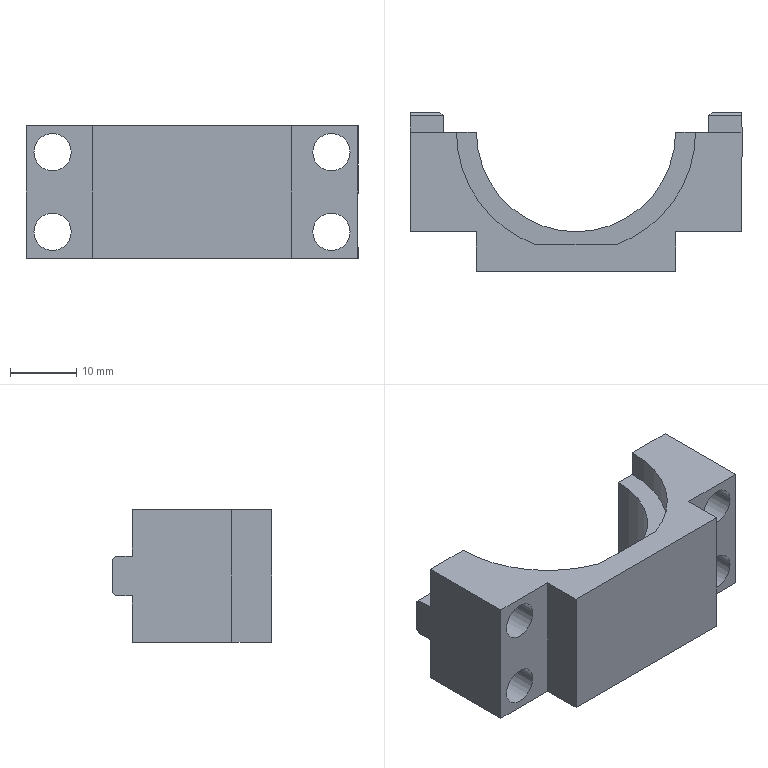Part | SolidWorks | features ICE 5, Chamfer 1, Extrusion 1 | 1 solid | 38 faces | box 50 x 24 x 20 mm | volume 9639 mm3 | plane 27 | cylinder 11 | commonest cylinder face diameters 5.6 x8 36 x2 30 x1
STEP:
#1=CARTESIAN_POINT('',(18.2,10.5,16.));
#2=VERTEX_POINT('',#1);
#3=CARTESIAN_POINT('',(23.8,10.5,16.));
#4=VERTEX_POINT('',#3);
#5=CARTESIAN_POINT('',(21.,10.5,16.));
#6=DIRECTION('',(0.,-1.,0.));
#7=DIRECTION('',(1.,0.,0.));
#8=AXIS2_PLACEMENT_3D('',#5,#6,#7);
#9=CIRCLE('',#8,2.8);
#10=EDGE_CURVE('',#2,#4,#9,.T.);
#11=ORIENTED_EDGE('',*,*,#10,.F.);
#12=CARTESIAN_POINT('',(18.2,-4.5,16.));
#13=VERTEX_POINT('',#12);
#14=CARTESIAN_POINT('',(18.2,15.5,16.));
#15=DIRECTION('',(0.,-1.,0.));
#16=VECTOR('',#15,1000.);
#17=LINE('',#14,#16);
#18=EDGE_CURVE('',#2,#13,#17,.T.);
#19=ORIENTED_EDGE('',*,*,#18,.T.);
#20=CARTESIAN_POINT('',(23.8,-4.5,16.));
#21=VERTEX_POINT('',#20);
#22=CARTESIAN_POINT('',(21.,-4.5,16.));
#23=DIRECTION('',(0.,-1.,0.));
#24=DIRECTION('',(1.,0.,0.));
#25=AXIS2_PLACEMENT_3D('',#22,#23,#24);
#26=CIRCLE('',#25,2.8);
#27=EDGE_CURVE('',#13,#21,#26,.T.);
#28=ORIENTED_EDGE('',*,*,#27,.T.);
#29=CARTESIAN_POINT('',(23.8,15.5,16.));
#30=DIRECTION('',(0.,-1.,0.));
#31=VECTOR('',#30,1000.);
#32=LINE('',#29,#31);
#33=EDGE_CURVE('',#4,#21,#32,.T.);
#34=ORIENTED_EDGE('',*,*,#33,.F.);
#35=EDGE_LOOP('',(#11,#19,#28,#34));
#36=FACE_OUTER_BOUND('',#35,.T.);
#37=CARTESIAN_POINT('',(21.,15.5,16.));
#38=DIRECTION('',(0.,-1.,0.));
#39=DIRECTION('',(1.,0.,0.));
#40=AXIS2_PLACEMENT_3D('',#37,#38,#39);
#41=CYLINDRICAL_SURFACE('',#40,2.8);
#42=ADVANCED_FACE('',(#36),#41,.F.);
#43=CARTESIAN_POINT('',(18.2,10.5,4.));
#44=VERTEX_POINT('',#43);
#45=CARTESIAN_POINT('',(23.8,10.5,4.));
#46=VERTEX_POINT('',#45);
#47=CARTESIAN_POINT('',(21.,10.5,4.));
#48=DIRECTION('',(0.,-1.,0.));
#49=DIRECTION('',(1.,0.,0.));
#50=AXIS2_PLACEMENT_3D('',#47,#48,#49);
#51=CIRCLE('',#50,2.8);
#52=EDGE_CURVE('',#44,#46,#51,.T.);
#53=ORIENTED_EDGE('',*,*,#52,.F.);
#54=CARTESIAN_POINT('',(18.2,-4.5,4.));
#55=VERTEX_POINT('',#54);
#56=CARTESIAN_POINT('',(18.2,15.5,4.));
#57=DIRECTION('',(0.,-1.,0.));
#58=VECTOR('',#57,1000.);
#59=LINE('',#56,#58);
#60=EDGE_CURVE('',#44,#55,#59,.T.);
#61=ORIENTED_EDGE('',*,*,#60,.T.);
#62=CARTESIAN_POINT('',(23.8,-4.5,4.));
#63=VERTEX_POINT('',#62);
#64=CARTESIAN_POINT('',(21.,-4.5,4.));
#65=DIRECTION('',(0.,-1.,0.));
#66=DIRECTION('',(1.,0.,0.));
#67=AXIS2_PLACEMENT_3D('',#64,#65,#66);
#68=CIRCLE('',#67,2.8);
#69=EDGE_CURVE('',#55,#63,#68,.T.);
#70=ORIENTED_EDGE('',*,*,#69,.T.);
#71=CARTESIAN_POINT('',(23.8,15.5,4.));
#72=DIRECTION('',(0.,-1.,0.));
#73=VECTOR('',#72,1000.);
#74=LINE('',#71,#73);
#75=EDGE_CURVE('',#46,#63,#74,.T.);
#76=ORIENTED_EDGE('',*,*,#75,.F.);
#77=EDGE_LOOP('',(#53,#61,#70,#76));
#78=FACE_OUTER_BOUND('',#77,.T.);
#79=CARTESIAN_POINT('',(21.,15.5,4.));
#80=DIRECTION('',(0.,-1.,0.));
#81=DIRECTION('',(1.,0.,0.));
#82=AXIS2_PLACEMENT_3D('',#79,#80,#81);
#83=CYLINDRICAL_SURFACE('',#82,2.8);
#84=ADVANCED_FACE('',(#78),#83,.F.);
#85=CARTESIAN_POINT('',(-23.8,10.5,4.));
#86=VERTEX_POINT('',#85);
#87=CARTESIAN_POINT('',(-18.2,10.5,4.));
#88=VERTEX_POINT('',#87);
#89=CARTESIAN_POINT('',(-21.,10.5,4.));
#90=DIRECTION('',(0.,-1.,0.));
#91=DIRECTION('',(1.,0.,0.));
#92=AXIS2_PLACEMENT_3D('',#89,#90,#91);
#93=CIRCLE('',#92,2.8);
#94=EDGE_CURVE('',#86,#88,#93,.T.);
#95=ORIENTED_EDGE('',*,*,#94,.F.);
#96=CARTESIAN_POINT('',(-23.8,-4.5,4.));
#97=VERTEX_POINT('',#96);
#98=CARTESIAN_POINT('',(-23.8,15.5,4.));
#99=DIRECTION('',(0.,-1.,0.));
#100=VECTOR('',#99,1000.);
#101=LINE('',#98,#100);
#102=EDGE_CURVE('',#86,#97,#101,.T.);
#103=ORIENTED_EDGE('',*,*,#102,.T.);
#104=CARTESIAN_POINT('',(-18.2,-4.5,4.));
#105=VERTEX_POINT('',#104);
#106=CARTESIAN_POINT('',(-21.,-4.5,4.));
#107=DIRECTION('',(0.,-1.,0.));
#108=DIRECTION('',(1.,0.,0.));
#109=AXIS2_PLACEMENT_3D('',#106,#107,#108);
#110=CIRCLE('',#109,2.8);
#111=EDGE_CURVE('',#97,#105,#110,.T.);
#112=ORIENTED_EDGE('',*,*,#111,.T.);
#113=CARTESIAN_POINT('',(-18.2,15.5,4.));
#114=DIRECTION('',(0.,-1.,0.));
#115=VECTOR('',#114,1000.);
#116=LINE('',#113,#115);
#117=EDGE_CURVE('',#88,#105,#116,.T.);
#118=ORIENTED_EDGE('',*,*,#117,.F.);
#119=EDGE_LOOP('',(#95,#103,#112,#118));
#120=FACE_OUTER_BOUND('',#119,.T.);
#121=CARTESIAN_POINT('',(-21.,15.5,4.));
#122=DIRECTION('',(0.,-1.,0.));
#123=DIRECTION('',(1.,0.,0.));
#124=AXIS2_PLACEMENT_3D('',#121,#122,#123);
#125=CYLINDRICAL_SURFACE('',#124,2.8);
#126=ADVANCED_FACE('',(#120),#125,.F.);
#127=CARTESIAN_POINT('',(-23.8,10.5,16.));
#128=VERTEX_POINT('',#127);
#129=CARTESIAN_POINT('',(-18.2,10.5,16.));
#130=VERTEX_POINT('',#129);
#131=CARTESIAN_POINT('',(-21.,10.5,16.));
#132=DIRECTION('',(0.,-1.,0.));
#133=DIRECTION('',(1.,0.,0.));
#134=AXIS2_PLACEMENT_3D('',#131,#132,#133);
#135=CIRCLE('',#134,2.8);
#136=EDGE_CURVE('',#128,#130,#135,.T.);
#137=ORIENTED_EDGE('',*,*,#136,.F.);
#138=CARTESIAN_POINT('',(-23.8,-4.5,16.));
#139=VERTEX_POINT('',#138);
#140=CARTESIAN_POINT('',(-23.8,15.5,16.));
#141=DIRECTION('',(0.,-1.,0.));
#142=VECTOR('',#141,1000.);
#143=LINE('',#140,#142);
#144=EDGE_CURVE('',#128,#139,#143,.T.);
#145=ORIENTED_EDGE('',*,*,#144,.T.);
#146=CARTESIAN_POINT('',(-18.2,-4.5,16.));
#147=VERTEX_POINT('',#146);
#148=CARTESIAN_POINT('',(-21.,-4.5,16.));
#149=DIRECTION('',(0.,-1.,0.));
#150=DIRECTION('',(1.,0.,0.));
#151=AXIS2_PLACEMENT_3D('',#148,#149,#150);
#152=CIRCLE('',#151,2.8);
#153=EDGE_CURVE('',#139,#147,#152,.T.);
#154=ORIENTED_EDGE('',*,*,#153,.T.);
#155=CARTESIAN_POINT('',(-18.2,15.5,16.));
#156=DIRECTION('',(0.,-1.,0.));
#157=VECTOR('',#156,1000.);
#158=LINE('',#155,#157);
#159=EDGE_CURVE('',#130,#147,#158,.T.);
#160=ORIENTED_EDGE('',*,*,#159,.F.);
#161=EDGE_LOOP('',(#137,#145,#154,#160));
#162=FACE_OUTER_BOUND('',#161,.T.);
#163=CARTESIAN_POINT('',(-21.,15.5,16.));
#164=DIRECTION('',(0.,-1.,0.));
#165=DIRECTION('',(1.,0.,0.));
#166=AXIS2_PLACEMENT_3D('',#163,#164,#165);
#167=CYLINDRICAL_SURFACE('',#166,2.8);
#168=ADVANCED_FACE('',(#162),#167,.F.);
#169=CARTESIAN_POINT('',(15.,10.5,16.));
#170=VERTEX_POINT('',#169);
#171=CARTESIAN_POINT('',(-15.,10.5,16.));
#172=VERTEX_POINT('',#171);
#173=CARTESIAN_POINT('',(0.,10.5,16.));
#174=DIRECTION('',(0.,0.,-1.));
#175=DIRECTION('',(1.,0.,0.));
#176=AXIS2_PLACEMENT_3D('',#173,#174,#175);
#177=CIRCLE('',#176,15.);
#178=EDGE_CURVE('',#170,#172,#177,.T.);
#179=ORIENTED_EDGE('',*,*,#178,.F.);
#180=CARTESIAN_POINT('',(15.,10.5,0.));
#181=VERTEX_POINT('',#180);
#182=CARTESIAN_POINT('',(15.,10.5,0.));
#183=DIRECTION('',(0.,0.,1.));
#184=VECTOR('',#183,1000.);
#185=LINE('',#182,#184);
#186=EDGE_CURVE('',#181,#170,#185,.T.);
#187=ORIENTED_EDGE('',*,*,#186,.F.);
#188=CARTESIAN_POINT('',(-15.,10.5,0.));
#189=VERTEX_POINT('',#188);
#190=CARTESIAN_POINT('',(0.,10.5,0.));
#191=DIRECTION('',(0.,0.,1.));
#192=DIRECTION('',(1.,0.,0.));
#193=AXIS2_PLACEMENT_3D('',#190,#191,#192);
#194=CIRCLE('',#193,15.);
#195=EDGE_CURVE('',#189,#181,#194,.T.);
#196=ORIENTED_EDGE('',*,*,#195,.F.);
#197=CARTESIAN_POINT('',(-15.,10.5,0.));
#198=DIRECTION('',(0.,0.,-1.));
#199=VECTOR('',#198,1000.);
#200=LINE('',#197,#199);
#201=EDGE_CURVE('',#172,#189,#200,.T.);
#202=ORIENTED_EDGE('',*,*,#201,.F.);
#203=EDGE_LOOP('',(#179,#187,#196,#202));
#204=FACE_OUTER_BOUND('',#203,.T.);
#205=CARTESIAN_POINT('',(0.,10.5,0.));
#206=DIRECTION('',(0.,0.,1.));
#207=DIRECTION('',(1.,0.,0.));
#208=AXIS2_PLACEMENT_3D('',#205,#206,#207);
#209=CYLINDRICAL_SURFACE('',#208,15.);
#210=ADVANCED_FACE('',(#204),#209,.F.);
#211=CARTESIAN_POINT('',(21.,10.5,4.));
#212=DIRECTION('',(0.,-1.,0.));
#213=DIRECTION('',(1.,0.,0.));
#214=AXIS2_PLACEMENT_3D('',#211,#212,#213);
#215=CIRCLE('',#214,2.8);
#216=EDGE_CURVE('',#46,#44,#215,.T.);
#217=ORIENTED_EDGE('',*,*,#216,.T.);
#218=ORIENTED_EDGE('',*,*,#52,.T.);
#219=EDGE_LOOP('',(#217,#218));
#220=FACE_BOUND('',#219,.T.);
#221=CARTESIAN_POINT('',(21.,10.5,16.));
#222=DIRECTION('',(0.,-1.,0.));
#223=DIRECTION('',(1.,0.,0.));
#224=AXIS2_PLACEMENT_3D('',#221,#222,#223);
#225=CIRCLE('',#224,2.8);
#226=EDGE_CURVE('',#4,#2,#225,.T.);
#227=ORIENTED_EDGE('',*,*,#226,.T.);
#228=ORIENTED_EDGE('',*,*,#10,.T.);
#229=EDGE_LOOP('',(#227,#228));
#230=FACE_BOUND('',#229,.T.);
#231=CARTESIAN_POINT('',(18.,10.5,16.));
#232=VERTEX_POINT('',#231);
#233=CARTESIAN_POINT('',(25.,10.5,16.));
#234=DIRECTION('',(-1.,0.,0.));
#235=VECTOR('',#234,1000.);
#236=LINE('',#233,#235);
#237=EDGE_CURVE('',#232,#170,#236,.T.);
#238=ORIENTED_EDGE('',*,*,#237,.F.);
#239=CARTESIAN_POINT('',(18.,10.5,20.));
#240=VERTEX_POINT('',#239);
#241=CARTESIAN_POINT('',(18.,10.5,16.));
#242=DIRECTION('',(0.,0.,1.));
#243=VECTOR('',#242,1000.);
#244=LINE('',#241,#243);
#245=EDGE_CURVE('',#232,#240,#244,.T.);
#246=ORIENTED_EDGE('',*,*,#245,.T.);
#247=CARTESIAN_POINT('',(25.,10.5,20.));
#248=VERTEX_POINT('',#247);
#249=CARTESIAN_POINT('',(25.,10.5,20.));
#250=DIRECTION('',(-1.,0.,0.));
#251=VECTOR('',#250,1000.);
#252=LINE('',#249,#251);
#253=EDGE_CURVE('',#248,#240,#252,.T.);
#254=ORIENTED_EDGE('',*,*,#253,.F.);
#255=CARTESIAN_POINT('',(25.,10.5,13.));
#256=VERTEX_POINT('',#255);
#257=CARTESIAN_POINT('',(25.,10.5,20.));
#258=DIRECTION('',(0.,0.,-1.));
#259=VECTOR('',#258,1000.);
#260=LINE('',#257,#259);
#261=EDGE_CURVE('',#248,#256,#260,.T.);
#262=ORIENTED_EDGE('',*,*,#261,.T.);
#263=CARTESIAN_POINT('',(20.,10.5,13.));
#264=VERTEX_POINT('',#263);
#265=CARTESIAN_POINT('',(20.,10.5,13.));
#266=DIRECTION('',(1.,0.,0.));
#267=VECTOR('',#266,1000.);
#268=LINE('',#265,#267);
#269=EDGE_CURVE('',#264,#256,#268,.T.);
#270=ORIENTED_EDGE('',*,*,#269,.F.);
#271=CARTESIAN_POINT('',(20.,10.5,7.));
#272=VERTEX_POINT('',#271);
#273=CARTESIAN_POINT('',(20.,10.5,13.));
#274=DIRECTION('',(0.,0.,1.));
#275=VECTOR('',#274,1000.);
#276=LINE('',#273,#275);
#277=EDGE_CURVE('',#272,#264,#276,.T.);
#278=ORIENTED_EDGE('',*,*,#277,.F.);
#279=CARTESIAN_POINT('',(25.,10.5,7.));
#280=VERTEX_POINT('',#279);
#281=CARTESIAN_POINT('',(20.,10.5,7.));
#282=DIRECTION('',(-1.,0.,0.));
#283=VECTOR('',#282,1000.);
#284=LINE('',#281,#283);
#285=EDGE_CURVE('',#280,#272,#284,.T.);
#286=ORIENTED_EDGE('',*,*,#285,.F.);
#287=CARTESIAN_POINT('',(25.,10.5,0.));
#288=VERTEX_POINT('',#287);
#289=CARTESIAN_POINT('',(25.,10.5,20.));
#290=DIRECTION('',(0.,0.,-1.));
#291=VECTOR('',#290,1000.);
#292=LINE('',#289,#291);
#293=EDGE_CURVE('',#280,#288,#292,.T.);
#294=ORIENTED_EDGE('',*,*,#293,.T.);
#295=CARTESIAN_POINT('',(25.,10.5,0.));
#296=DIRECTION('',(-1.,0.,0.));
#297=VECTOR('',#296,1000.);
#298=LINE('',#295,#297);
#299=EDGE_CURVE('',#288,#181,#298,.T.);
#300=ORIENTED_EDGE('',*,*,#299,.T.);
#301=ORIENTED_EDGE('',*,*,#186,.T.);
#302=EDGE_LOOP('',(#238,#246,#254,#262,#270,#278,#286,#294,#300,#301));
#303=FACE_OUTER_BOUND('',#302,.T.);
#304=CARTESIAN_POINT('',(25.,10.5,20.));
#305=DIRECTION('',(0.,-1.,0.));
#306=DIRECTION('',(1.,0.,0.));
#307=AXIS2_PLACEMENT_3D('',#304,#305,#306);
#308=PLANE('',#307);
#309=ADVANCED_FACE('',(#220,#230,#303),#308,.F.);
#310=CARTESIAN_POINT('',(-21.,10.5,16.));
#311=DIRECTION('',(0.,-1.,0.));
#312=DIRECTION('',(1.,0.,0.));
#313=AXIS2_PLACEMENT_3D('',#310,#311,#312);
#314=CIRCLE('',#313,2.8);
#315=EDGE_CURVE('',#130,#128,#314,.T.);
#316=ORIENTED_EDGE('',*,*,#315,.T.);
#317=ORIENTED_EDGE('',*,*,#136,.T.);
#318=EDGE_LOOP('',(#316,#317));
#319=FACE_BOUND('',#318,.T.);
#320=CARTESIAN_POINT('',(-21.,10.5,4.));
#321=DIRECTION('',(0.,-1.,0.));
#322=DIRECTION('',(1.,0.,0.));
#323=AXIS2_PLACEMENT_3D('',#320,#321,#322);
#324=CIRCLE('',#323,2.8);
#325=EDGE_CURVE('',#88,#86,#324,.T.);
#326=ORIENTED_EDGE('',*,*,#325,.T.);
#327=ORIENTED_EDGE('',*,*,#94,.T.);
#328=EDGE_LOOP('',(#326,#327));
#329=FACE_BOUND('',#328,.T.);
#330=CARTESIAN_POINT('',(-18.,10.5,20.));
#331=VERTEX_POINT('',#330);
#332=CARTESIAN_POINT('',(-25.,10.5,20.));
#333=VERTEX_POINT('',#332);
#334=CARTESIAN_POINT('',(25.,10.5,20.));
#335=DIRECTION('',(-1.,0.,0.));
#336=VECTOR('',#335,1000.);
#337=LINE('',#334,#336);
#338=EDGE_CURVE('',#331,#333,#337,.T.);
#339=ORIENTED_EDGE('',*,*,#338,.F.);
#340=CARTESIAN_POINT('',(-18.,10.5,16.));
#341=VERTEX_POINT('',#340);
#342=CARTESIAN_POINT('',(-18.,10.5,16.));
#343=DIRECTION('',(0.,0.,-1.));
#344=VECTOR('',#343,1000.);
#345=LINE('',#342,#344);
#346=EDGE_CURVE('',#331,#341,#345,.T.);
#347=ORIENTED_EDGE('',*,*,#346,.T.);
#348=CARTESIAN_POINT('',(25.,10.5,16.));
#349=DIRECTION('',(-1.,0.,0.));
#350=VECTOR('',#349,1000.);
#351=LINE('',#348,#350);
#352=EDGE_CURVE('',#172,#341,#351,.T.);
#353=ORIENTED_EDGE('',*,*,#352,.F.);
#354=ORIENTED_EDGE('',*,*,#201,.T.);
#355=CARTESIAN_POINT('',(-25.,10.5,0.));
#356=VERTEX_POINT('',#355);
#357=CARTESIAN_POINT('',(25.,10.5,0.));
#358=DIRECTION('',(-1.,0.,0.));
#359=VECTOR('',#358,1000.);
#360=LINE('',#357,#359);
#361=EDGE_CURVE('',#189,#356,#360,.T.);
#362=ORIENTED_EDGE('',*,*,#361,.T.);
#363=CARTESIAN_POINT('',(-25.,10.5,7.));
#364=VERTEX_POINT('',#363);
#365=CARTESIAN_POINT('',(-25.,10.5,20.));
#366=DIRECTION('',(0.,0.,-1.));
#367=VECTOR('',#366,1000.);
#368=LINE('',#365,#367);
#369=EDGE_CURVE('',#364,#356,#368,.T.);
#370=ORIENTED_EDGE('',*,*,#369,.F.);
#371=CARTESIAN_POINT('',(-20.,10.5,7.));
#372=VERTEX_POINT('',#371);
#373=CARTESIAN_POINT('',(-20.,10.5,7.));
#374=DIRECTION('',(-1.,0.,0.));
#375=VECTOR('',#374,1000.);
#376=LINE('',#373,#375);
#377=EDGE_CURVE('',#372,#364,#376,.T.);
#378=ORIENTED_EDGE('',*,*,#377,.F.);
#379=CARTESIAN_POINT('',(-20.,10.5,13.));
#380=VERTEX_POINT('',#379);
#381=CARTESIAN_POINT('',(-20.,10.5,13.));
#382=DIRECTION('',(0.,0.,-1.));
#383=VECTOR('',#382,1000.);
#384=LINE('',#381,#383);
#385=EDGE_CURVE('',#380,#372,#384,.T.);
#386=ORIENTED_EDGE('',*,*,#385,.F.);
#387=CARTESIAN_POINT('',(-25.,10.5,13.));
#388=VERTEX_POINT('',#387);
#389=CARTESIAN_POINT('',(-20.,10.5,13.));
#390=DIRECTION('',(1.,0.,0.));
#391=VECTOR('',#390,1000.);
#392=LINE('',#389,#391);
#393=EDGE_CURVE('',#388,#380,#392,.T.);
#394=ORIENTED_EDGE('',*,*,#393,.F.);
#395=CARTESIAN_POINT('',(-25.,10.5,20.));
#396=DIRECTION('',(0.,0.,-1.));
#397=VECTOR('',#396,1000.);
#398=LINE('',#395,#397);
#399=EDGE_CURVE('',#333,#388,#398,.T.);
#400=ORIENTED_EDGE('',*,*,#399,.F.);
#401=EDGE_LOOP('',(#339,#347,#353,#354,#362,#370,#378,#386,#394,#400));
#402=FACE_OUTER_BOUND('',#401,.T.);
#403=CARTESIAN_POINT('',(25.,10.5,20.));
#404=DIRECTION('',(0.,-1.,0.));
#405=DIRECTION('',(1.,0.,0.));
#406=AXIS2_PLACEMENT_3D('',#403,#404,#405);
#407=PLANE('',#406);
#408=ADVANCED_FACE('',(#319,#329,#402),#407,.F.);
#409=CARTESIAN_POINT('',(-15.,-10.5,0.));
#410=VERTEX_POINT('',#409);
#411=CARTESIAN_POINT('',(-15.,-10.5,20.));
#412=VERTEX_POINT('',#411);
#413=CARTESIAN_POINT('',(-15.,-10.5,0.));
#414=DIRECTION('',(0.,0.,1.));
#415=VECTOR('',#414,1000.);
#416=LINE('',#413,#415);
#417=EDGE_CURVE('',#410,#412,#416,.T.);
#418=ORIENTED_EDGE('',*,*,#417,.F.);
#419=CARTESIAN_POINT('',(15.,-10.5,0.));
#420=VERTEX_POINT('',#419);
#421=CARTESIAN_POINT('',(25.,-10.5,0.));
#422=DIRECTION('',(-1.,0.,0.));
#423=VECTOR('',#422,1000.);
#424=LINE('',#421,#423);
#425=EDGE_CURVE('',#420,#410,#424,.T.);
#426=ORIENTED_EDGE('',*,*,#425,.F.);
#427=CARTESIAN_POINT('',(15.,-10.5,20.));
#428=VERTEX_POINT('',#427);
#429=CARTESIAN_POINT('',(15.,-10.5,0.));
#430=DIRECTION('',(0.,0.,1.));
#431=VECTOR('',#430,1000.);
#432=LINE('',#429,#431);
#433=EDGE_CURVE('',#420,#428,#432,.T.);
#434=ORIENTED_EDGE('',*,*,#433,.T.);
#435=CARTESIAN_POINT('',(25.,-10.5,20.));
#436=DIRECTION('',(-1.,0.,0.));
#437=VECTOR('',#436,1000.);
#438=LINE('',#435,#437);
#439=EDGE_CURVE('',#428,#412,#438,.T.);
#440=ORIENTED_EDGE('',*,*,#439,.T.);
#441=EDGE_LOOP('',(#418,#426,#434,#440));
#442=FACE_OUTER_BOUND('',#441,.T.);
#443=CARTESIAN_POINT('',(25.,-10.5,20.));
#444=DIRECTION('',(0.,-1.,0.));
#445=DIRECTION('',(1.,0.,0.));
#446=AXIS2_PLACEMENT_3D('',#443,#444,#445);
#447=PLANE('',#446);
#448=ADVANCED_FACE('',(#442),#447,.T.);
#449=CARTESIAN_POINT('',(25.,13.5,12.5));
#450=VERTEX_POINT('',#449);
#451=CARTESIAN_POINT('',(25.,13.5,7.5));
#452=VERTEX_POINT('',#451);
#453=CARTESIAN_POINT('',(25.,13.5,13.));
#454=DIRECTION('',(0.,0.,-1.));
#455=VECTOR('',#454,1000.);
#456=LINE('',#453,#455);
#457=EDGE_CURVE('',#450,#452,#456,.T.);
#458=ORIENTED_EDGE('',*,*,#457,.F.);
#459=CARTESIAN_POINT('',(25.,13.,13.));
#460=VERTEX_POINT('',#459);
#461=CARTESIAN_POINT('',(25.,8.25,17.75));
#462=DIRECTION('',(0.,-0.7071,0.7071));
#463=VECTOR('',#462,1000.);
#464=LINE('',#461,#463);
#465=EDGE_CURVE('',#450,#460,#464,.T.);
#466=ORIENTED_EDGE('',*,*,#465,.T.);
#467=CARTESIAN_POINT('',(25.,13.5,13.));
#468=DIRECTION('',(0.,-1.,0.));
#469=VECTOR('',#468,1000.);
#470=LINE('',#467,#469);
#471=EDGE_CURVE('',#460,#256,#470,.T.);
#472=ORIENTED_EDGE('',*,*,#471,.T.);
#473=ORIENTED_EDGE('',*,*,#261,.F.);
#474=CARTESIAN_POINT('',(25.,-4.5,20.));
#475=VERTEX_POINT('',#474);
#476=CARTESIAN_POINT('',(25.,10.5,20.));
#477=DIRECTION('',(0.,-1.,0.));
#478=VECTOR('',#477,1000.);
#479=LINE('',#476,#478);
#480=EDGE_CURVE('',#248,#475,#479,.T.);
#481=ORIENTED_EDGE('',*,*,#480,.T.);
#482=CARTESIAN_POINT('',(25.,-4.5,0.));
#483=VERTEX_POINT('',#482);
#484=CARTESIAN_POINT('',(25.,-4.5,0.));
#485=DIRECTION('',(0.,0.,1.));
#486=VECTOR('',#485,1000.);
#487=LINE('',#484,#486);
#488=EDGE_CURVE('',#483,#475,#487,.T.);
#489=ORIENTED_EDGE('',*,*,#488,.F.);
#490=CARTESIAN_POINT('',(25.,10.5,0.));
#491=DIRECTION('',(0.,-1.,0.));
#492=VECTOR('',#491,1000.);
#493=LINE('',#490,#492);
#494=EDGE_CURVE('',#288,#483,#493,.T.);
#495=ORIENTED_EDGE('',*,*,#494,.F.);
#496=ORIENTED_EDGE('',*,*,#293,.F.);
#497=CARTESIAN_POINT('',(25.,13.,7.));
#498=VERTEX_POINT('',#497);
#499=CARTESIAN_POINT('',(25.,13.5,7.));
#500=DIRECTION('',(0.,-1.,0.));
#501=VECTOR('',#500,1000.);
#502=LINE('',#499,#501);
#503=EDGE_CURVE('',#498,#280,#502,.T.);
#504=ORIENTED_EDGE('',*,*,#503,.F.);
#505=CARTESIAN_POINT('',(25.,18.25,12.25));
#506=DIRECTION('',(0.,0.7071,0.7071));
#507=VECTOR('',#506,1000.);
#508=LINE('',#505,#507);
#509=EDGE_CURVE('',#498,#452,#508,.T.);
#510=ORIENTED_EDGE('',*,*,#509,.T.);
#511=EDGE_LOOP('',(#458,#466,#472,#473,#481,#489,#495,#496,#504,#510));
#512=FACE_OUTER_BOUND('',#511,.T.);
#513=CARTESIAN_POINT('',(25.,10.5,20.));
#514=DIRECTION('',(1.,0.,0.));
#515=DIRECTION('',(0.,1.,0.));
#516=AXIS2_PLACEMENT_3D('',#513,#514,#515);
#517=PLANE('',#516);
#518=ADVANCED_FACE('',(#512),#517,.T.);
#519=CARTESIAN_POINT('',(-25.,13.5,7.5));
#520=VERTEX_POINT('',#519);
#521=CARTESIAN_POINT('',(-25.,13.5,12.5));
#522=VERTEX_POINT('',#521);
#523=CARTESIAN_POINT('',(-25.,13.5,13.));
#524=DIRECTION('',(0.,0.,1.));
#525=VECTOR('',#524,1000.);
#526=LINE('',#523,#525);
#527=EDGE_CURVE('',#520,#522,#526,.T.);
#528=ORIENTED_EDGE('',*,*,#527,.F.);
#529=CARTESIAN_POINT('',(-25.,13.,7.));
#530=VERTEX_POINT('',#529);
#531=CARTESIAN_POINT('',(-25.,13.5,7.5));
#532=DIRECTION('',(0.,-0.7071,-0.7071));
#533=VECTOR('',#532,1000.);
#534=LINE('',#531,#533);
#535=EDGE_CURVE('',#520,#530,#534,.T.);
#536=ORIENTED_EDGE('',*,*,#535,.T.);
#537=CARTESIAN_POINT('',(-25.,13.5,7.));
#538=DIRECTION('',(0.,-1.,0.));
#539=VECTOR('',#538,1000.);
#540=LINE('',#537,#539);
#541=EDGE_CURVE('',#530,#364,#540,.T.);
#542=ORIENTED_EDGE('',*,*,#541,.T.);
#543=ORIENTED_EDGE('',*,*,#369,.T.);
#544=CARTESIAN_POINT('',(-25.,-4.5,0.));
#545=VERTEX_POINT('',#544);
#546=CARTESIAN_POINT('',(-25.,10.5,0.));
#547=DIRECTION('',(0.,-1.,0.));
#548=VECTOR('',#547,1000.);
#549=LINE('',#546,#548);
#550=EDGE_CURVE('',#356,#545,#549,.T.);
#551=ORIENTED_EDGE('',*,*,#550,.T.);
#552=CARTESIAN_POINT('',(-25.,-4.5,20.));
#553=VERTEX_POINT('',#552);
#554=CARTESIAN_POINT('',(-25.,-4.5,0.));
#555=DIRECTION('',(0.,0.,1.));
#556=VECTOR('',#555,1000.);
#557=LINE('',#554,#556);
#558=EDGE_CURVE('',#545,#553,#557,.T.);
#559=ORIENTED_EDGE('',*,*,#558,.T.);
#560=CARTESIAN_POINT('',(-25.,10.5,20.));
#561=DIRECTION('',(0.,-1.,0.));
#562=VECTOR('',#561,1000.);
#563=LINE('',#560,#562);
#564=EDGE_CURVE('',#333,#553,#563,.T.);
#565=ORIENTED_EDGE('',*,*,#564,.F.);
#566=ORIENTED_EDGE('',*,*,#399,.T.);
#567=CARTESIAN_POINT('',(-25.,13.,13.));
#568=VERTEX_POINT('',#567);
#569=CARTESIAN_POINT('',(-25.,13.5,13.));
#570=DIRECTION('',(0.,-1.,0.));
#571=VECTOR('',#570,1000.);
#572=LINE('',#569,#571);
#573=EDGE_CURVE('',#568,#388,#572,.T.);
#574=ORIENTED_EDGE('',*,*,#573,.F.);
#575=CARTESIAN_POINT('',(-25.,13.5,12.5));
#576=DIRECTION('',(0.,0.7071,-0.7071));
#577=VECTOR('',#576,1000.);
#578=LINE('',#575,#577);
#579=EDGE_CURVE('',#568,#522,#578,.T.);
#580=ORIENTED_EDGE('',*,*,#579,.T.);
#581=EDGE_LOOP('',(#528,#536,#542,#543,#551,#559,#565,#566,#574,#580));
#582=FACE_OUTER_BOUND('',#581,.T.);
#583=CARTESIAN_POINT('',(-25.,10.5,20.));
#584=DIRECTION('',(1.,0.,0.));
#585=DIRECTION('',(0.,1.,0.));
#586=AXIS2_PLACEMENT_3D('',#583,#584,#585);
#587=PLANE('',#586);
#588=ADVANCED_FACE('',(#582),#587,.F.);
#589=CARTESIAN_POINT('',(5.916,-6.5,20.));
#590=VERTEX_POINT('',#589);
#591=CARTESIAN_POINT('',(0.,10.5,20.));
#592=DIRECTION('',(0.,0.,1.));
#593=DIRECTION('',(1.,0.,0.));
#594=AXIS2_PLACEMENT_3D('',#591,#592,#593);
#595=CIRCLE('',#594,18.);
#596=EDGE_CURVE('',#590,#240,#595,.T.);
#597=ORIENTED_EDGE('',*,*,#596,.F.);
#598=CARTESIAN_POINT('',(-5.916,-6.5,20.));
#599=VERTEX_POINT('',#598);
#600=CARTESIAN_POINT('',(-5.916,-6.5,20.));
#601=DIRECTION('',(1.,0.,0.));
#602=VECTOR('',#601,1000.);
#603=LINE('',#600,#602);
#604=EDGE_CURVE('',#599,#590,#603,.T.);
#605=ORIENTED_EDGE('',*,*,#604,.F.);
#606=CARTESIAN_POINT('',(0.,10.5,20.));
#607=DIRECTION('',(0.,0.,1.));
#608=DIRECTION('',(1.,0.,0.));
#609=AXIS2_PLACEMENT_3D('',#606,#607,#608);
#610=CIRCLE('',#609,18.);
#611=EDGE_CURVE('',#331,#599,#610,.T.);
#612=ORIENTED_EDGE('',*,*,#611,.F.);
#613=ORIENTED_EDGE('',*,*,#338,.T.);
#614=ORIENTED_EDGE('',*,*,#564,.T.);
#615=CARTESIAN_POINT('',(-15.,-4.5,20.));
#616=VERTEX_POINT('',#615);
#617=CARTESIAN_POINT('',(-15.,-4.5,20.));
#618=DIRECTION('',(-1.,0.,0.));
#619=VECTOR('',#618,1000.);
#620=LINE('',#617,#619);
#621=EDGE_CURVE('',#616,#553,#620,.T.);
#622=ORIENTED_EDGE('',*,*,#621,.F.);
#623=CARTESIAN_POINT('',(-15.,-4.5,20.));
#624=DIRECTION('',(0.,1.,0.));
#625=VECTOR('',#624,1000.);
#626=LINE('',#623,#625);
#627=EDGE_CURVE('',#412,#616,#626,.T.);
#628=ORIENTED_EDGE('',*,*,#627,.F.);
#629=ORIENTED_EDGE('',*,*,#439,.F.);
#630=CARTESIAN_POINT('',(15.,-4.5,20.));
#631=VERTEX_POINT('',#630);
#632=CARTESIAN_POINT('',(15.,-4.5,20.));
#633=DIRECTION('',(0.,-1.,0.));
#634=VECTOR('',#633,1000.);
#635=LINE('',#632,#634);
#636=EDGE_CURVE('',#631,#428,#635,.T.);
#637=ORIENTED_EDGE('',*,*,#636,.F.);
#638=CARTESIAN_POINT('',(15.,-4.5,20.));
#639=DIRECTION('',(-1.,0.,0.));
#640=VECTOR('',#639,1000.);
#641=LINE('',#638,#640);
#642=EDGE_CURVE('',#475,#631,#641,.T.);
#643=ORIENTED_EDGE('',*,*,#642,.F.);
#644=ORIENTED_EDGE('',*,*,#480,.F.);
#645=ORIENTED_EDGE('',*,*,#253,.T.);
#646=EDGE_LOOP('',(#597,#605,#612,#613,#614,#622,#628,#629,#637,#643,#644,#645));
#647=FACE_OUTER_BOUND('',#646,.T.);
#648=CARTESIAN_POINT('',(0.,0.,20.));
#649=DIRECTION('',(0.,0.,1.));
#650=DIRECTION('',(1.,0.,0.));
#651=AXIS2_PLACEMENT_3D('',#648,#649,#650);
#652=PLANE('',#651);
#653=ADVANCED_FACE('',(#647),#652,.T.);
#654=CARTESIAN_POINT('',(-15.,-4.5,0.));
#655=VERTEX_POINT('',#654);
#656=CARTESIAN_POINT('',(-15.,-4.5,0.));
#657=DIRECTION('',(0.,1.,0.));
#658=VECTOR('',#657,1000.);
#659=LINE('',#656,#658);
#660=EDGE_CURVE('',#410,#655,#659,.T.);
#661=ORIENTED_EDGE('',*,*,#660,.T.);
#662=CARTESIAN_POINT('',(-15.,-4.5,0.));
#663=DIRECTION('',(-1.,0.,0.));
#664=VECTOR('',#663,1000.);
#665=LINE('',#662,#664);
#666=EDGE_CURVE('',#655,#545,#665,.T.);
#667=ORIENTED_EDGE('',*,*,#666,.T.);
#668=ORIENTED_EDGE('',*,*,#550,.F.);
#669=ORIENTED_EDGE('',*,*,#361,.F.);
#670=ORIENTED_EDGE('',*,*,#195,.T.);
#671=ORIENTED_EDGE('',*,*,#299,.F.);
#672=ORIENTED_EDGE('',*,*,#494,.T.);
#673=CARTESIAN_POINT('',(15.,-4.5,0.));
#674=VERTEX_POINT('',#673);
#675=CARTESIAN_POINT('',(15.,-4.5,0.));
#676=DIRECTION('',(-1.,0.,0.));
#677=VECTOR('',#676,1000.);
#678=LINE('',#675,#677);
#679=EDGE_CURVE('',#483,#674,#678,.T.);
#680=ORIENTED_EDGE('',*,*,#679,.T.);
#681=CARTESIAN_POINT('',(15.,-4.5,0.));
#682=DIRECTION('',(0.,-1.,0.));
#683=VECTOR('',#682,1000.);
#684=LINE('',#681,#683);
#685=EDGE_CURVE('',#674,#420,#684,.T.);
#686=ORIENTED_EDGE('',*,*,#685,.T.);
#687=ORIENTED_EDGE('',*,*,#425,.T.);
#688=EDGE_LOOP('',(#661,#667,#668,#669,#670,#671,#672,#680,#686,#687));
#689=FACE_OUTER_BOUND('',#688,.T.);
#690=CARTESIAN_POINT('',(0.,0.,0.));
#691=DIRECTION('',(0.,0.,1.));
#692=DIRECTION('',(1.,0.,0.));
#693=AXIS2_PLACEMENT_3D('',#690,#691,#692);
#694=PLANE('',#693);
#695=ADVANCED_FACE('',(#689),#694,.F.);
#696=ORIENTED_EDGE('',*,*,#636,.T.);
#697=ORIENTED_EDGE('',*,*,#433,.F.);
#698=ORIENTED_EDGE('',*,*,#685,.F.);
#699=CARTESIAN_POINT('',(15.,-4.5,0.));
#700=DIRECTION('',(0.,0.,1.));
#701=VECTOR('',#700,1000.);
#702=LINE('',#699,#701);
#703=EDGE_CURVE('',#674,#631,#702,.T.);
#704=ORIENTED_EDGE('',*,*,#703,.T.);
#705=EDGE_LOOP('',(#696,#697,#698,#704));
#706=FACE_OUTER_BOUND('',#705,.T.);
#707=CARTESIAN_POINT('',(15.,-4.5,0.));
#708=DIRECTION('',(-1.,0.,0.));
#709=DIRECTION('',(0.,-1.,0.));
#710=AXIS2_PLACEMENT_3D('',#707,#708,#709);
#711=PLANE('',#710);
#712=ADVANCED_FACE('',(#706),#711,.F.);
#713=CARTESIAN_POINT('',(21.,-4.5,16.));
#714=DIRECTION('',(0.,-1.,0.));
#715=DIRECTION('',(1.,0.,0.));
#716=AXIS2_PLACEMENT_3D('',#713,#714,#715);
#717=CIRCLE('',#716,2.8);
#718=EDGE_CURVE('',#21,#13,#717,.T.);
#719=ORIENTED_EDGE('',*,*,#718,.F.);
#720=ORIENTED_EDGE('',*,*,#27,.F.);
#721=EDGE_LOOP('',(#719,#720));
#722=FACE_BOUND('',#721,.T.);
#723=CARTESIAN_POINT('',(21.,-4.5,4.));
#724=DIRECTION('',(0.,-1.,0.));
#725=DIRECTION('',(1.,0.,0.));
#726=AXIS2_PLACEMENT_3D('',#723,#724,#725);
#727=CIRCLE('',#726,2.8);
#728=EDGE_CURVE('',#63,#55,#727,.T.);
#729=ORIENTED_EDGE('',*,*,#728,.F.);
#730=ORIENTED_EDGE('',*,*,#69,.F.);
#731=EDGE_LOOP('',(#729,#730));
#732=FACE_BOUND('',#731,.T.);
#733=ORIENTED_EDGE('',*,*,#642,.T.);
#734=ORIENTED_EDGE('',*,*,#703,.F.);
#735=ORIENTED_EDGE('',*,*,#679,.F.);
#736=ORIENTED_EDGE('',*,*,#488,.T.);
#737=EDGE_LOOP('',(#733,#734,#735,#736));
#738=FACE_OUTER_BOUND('',#737,.T.);
#739=CARTESIAN_POINT('',(15.,-4.5,0.));
#740=DIRECTION('',(0.,1.,0.));
#741=DIRECTION('',(-1.,0.,0.));
#742=AXIS2_PLACEMENT_3D('',#739,#740,#741);
#743=PLANE('',#742);
#744=ADVANCED_FACE('',(#722,#732,#738),#743,.F.);
#745=CARTESIAN_POINT('',(-21.,-4.5,4.));
#746=DIRECTION('',(0.,-1.,0.));
#747=DIRECTION('',(1.,0.,0.));
#748=AXIS2_PLACEMENT_3D('',#745,#746,#747);
#749=CIRCLE('',#748,2.8);
#750=EDGE_CURVE('',#105,#97,#749,.T.);
#751=ORIENTED_EDGE('',*,*,#750,.F.);
#752=ORIENTED_EDGE('',*,*,#111,.F.);
#753=EDGE_LOOP('',(#751,#752));
#754=FACE_BOUND('',#753,.T.);
#755=CARTESIAN_POINT('',(-21.,-4.5,16.));
#756=DIRECTION('',(0.,-1.,0.));
#757=DIRECTION('',(1.,0.,0.));
#758=AXIS2_PLACEMENT_3D('',#755,#756,#757);
#759=CIRCLE('',#758,2.8);
#760=EDGE_CURVE('',#147,#139,#759,.T.);
#761=ORIENTED_EDGE('',*,*,#760,.F.);
#762=ORIENTED_EDGE('',*,*,#153,.F.);
#763=EDGE_LOOP('',(#761,#762));
#764=FACE_BOUND('',#763,.T.);
#765=ORIENTED_EDGE('',*,*,#621,.T.);
#766=ORIENTED_EDGE('',*,*,#558,.F.);
#767=ORIENTED_EDGE('',*,*,#666,.F.);
#768=CARTESIAN_POINT('',(-15.,-4.5,0.));
#769=DIRECTION('',(0.,0.,1.));
#770=VECTOR('',#769,1000.);
#771=LINE('',#768,#770);
#772=EDGE_CURVE('',#655,#616,#771,.T.);
#773=ORIENTED_EDGE('',*,*,#772,.T.);
#774=EDGE_LOOP('',(#765,#766,#767,#773));
#775=FACE_OUTER_BOUND('',#774,.T.);
#776=CARTESIAN_POINT('',(-15.,-4.5,0.));
#777=DIRECTION('',(0.,1.,0.));
#778=DIRECTION('',(-1.,0.,0.));
#779=AXIS2_PLACEMENT_3D('',#776,#777,#778);
#780=PLANE('',#779);
#781=ADVANCED_FACE('',(#754,#764,#775),#780,.F.);
#782=ORIENTED_EDGE('',*,*,#627,.T.);
#783=ORIENTED_EDGE('',*,*,#772,.F.);
#784=ORIENTED_EDGE('',*,*,#660,.F.);
#785=ORIENTED_EDGE('',*,*,#417,.T.);
#786=EDGE_LOOP('',(#782,#783,#784,#785));
#787=FACE_OUTER_BOUND('',#786,.T.);
#788=CARTESIAN_POINT('',(-15.,-4.5,0.));
#789=DIRECTION('',(1.,0.,0.));
#790=DIRECTION('',(0.,1.,0.));
#791=AXIS2_PLACEMENT_3D('',#788,#789,#790);
#792=PLANE('',#791);
#793=ADVANCED_FACE('',(#787),#792,.F.);
#794=ORIENTED_EDGE('',*,*,#144,.F.);
#795=ORIENTED_EDGE('',*,*,#315,.F.);
#796=ORIENTED_EDGE('',*,*,#159,.T.);
#797=ORIENTED_EDGE('',*,*,#760,.T.);
#798=EDGE_LOOP('',(#794,#795,#796,#797));
#799=FACE_OUTER_BOUND('',#798,.T.);
#800=CARTESIAN_POINT('',(-21.,15.5,16.));
#801=DIRECTION('',(0.,-1.,0.));
#802=DIRECTION('',(1.,0.,0.));
#803=AXIS2_PLACEMENT_3D('',#800,#801,#802);
#804=CYLINDRICAL_SURFACE('',#803,2.8);
#805=ADVANCED_FACE('',(#799),#804,.F.);
#806=ORIENTED_EDGE('',*,*,#102,.F.);
#807=ORIENTED_EDGE('',*,*,#325,.F.);
#808=ORIENTED_EDGE('',*,*,#117,.T.);
#809=ORIENTED_EDGE('',*,*,#750,.T.);
#810=EDGE_LOOP('',(#806,#807,#808,#809));
#811=FACE_OUTER_BOUND('',#810,.T.);
#812=CARTESIAN_POINT('',(-21.,15.5,4.));
#813=DIRECTION('',(0.,-1.,0.));
#814=DIRECTION('',(1.,0.,0.));
#815=AXIS2_PLACEMENT_3D('',#812,#813,#814);
#816=CYLINDRICAL_SURFACE('',#815,2.8);
#817=ADVANCED_FACE('',(#811),#816,.F.);
#818=ORIENTED_EDGE('',*,*,#60,.F.);
#819=ORIENTED_EDGE('',*,*,#216,.F.);
#820=ORIENTED_EDGE('',*,*,#75,.T.);
#821=ORIENTED_EDGE('',*,*,#728,.T.);
#822=EDGE_LOOP('',(#818,#819,#820,#821));
#823=FACE_OUTER_BOUND('',#822,.T.);
#824=CARTESIAN_POINT('',(21.,15.5,4.));
#825=DIRECTION('',(0.,-1.,0.));
#826=DIRECTION('',(1.,0.,0.));
#827=AXIS2_PLACEMENT_3D('',#824,#825,#826);
#828=CYLINDRICAL_SURFACE('',#827,2.8);
#829=ADVANCED_FACE('',(#823),#828,.F.);
#830=ORIENTED_EDGE('',*,*,#18,.F.);
#831=ORIENTED_EDGE('',*,*,#226,.F.);
#832=ORIENTED_EDGE('',*,*,#33,.T.);
#833=ORIENTED_EDGE('',*,*,#718,.T.);
#834=EDGE_LOOP('',(#830,#831,#832,#833));
#835=FACE_OUTER_BOUND('',#834,.T.);
#836=CARTESIAN_POINT('',(21.,15.5,16.));
#837=DIRECTION('',(0.,-1.,0.));
#838=DIRECTION('',(1.,0.,0.));
#839=AXIS2_PLACEMENT_3D('',#836,#837,#838);
#840=CYLINDRICAL_SURFACE('',#839,2.8);
#841=ADVANCED_FACE('',(#835),#840,.F.);
#842=CARTESIAN_POINT('',(-20.,13.,13.));
#843=VERTEX_POINT('',#842);
#844=CARTESIAN_POINT('',(-20.,13.5,13.));
#845=DIRECTION('',(0.,-1.,0.));
#846=VECTOR('',#845,1000.);
#847=LINE('',#844,#846);
#848=EDGE_CURVE('',#843,#380,#847,.T.);
#849=ORIENTED_EDGE('',*,*,#848,.F.);
#850=CARTESIAN_POINT('',(-25.,13.,13.));
#851=DIRECTION('',(-1.,0.,0.));
#852=VECTOR('',#851,1000.);
#853=LINE('',#850,#852);
#854=EDGE_CURVE('',#843,#568,#853,.T.);
#855=ORIENTED_EDGE('',*,*,#854,.T.);
#856=ORIENTED_EDGE('',*,*,#573,.T.);
#857=ORIENTED_EDGE('',*,*,#393,.T.);
#858=EDGE_LOOP('',(#849,#855,#856,#857));
#859=FACE_OUTER_BOUND('',#858,.T.);
#860=CARTESIAN_POINT('',(-20.,13.5,13.));
#861=DIRECTION('',(0.,0.,-1.));
#862=DIRECTION('',(-1.,0.,0.));
#863=AXIS2_PLACEMENT_3D('',#860,#861,#862);
#864=PLANE('',#863);
#865=ADVANCED_FACE('',(#859),#864,.F.);
#866=CARTESIAN_POINT('',(-20.,13.,7.));
#867=VERTEX_POINT('',#866);
#868=CARTESIAN_POINT('',(-20.,13.5,7.));
#869=DIRECTION('',(0.,-1.,0.));
#870=VECTOR('',#869,1000.);
#871=LINE('',#868,#870);
#872=EDGE_CURVE('',#867,#372,#871,.T.);
#873=ORIENTED_EDGE('',*,*,#872,.F.);
#874=CARTESIAN_POINT('',(-20.,13.,13.));
#875=DIRECTION('',(0.,0.,1.));
#876=VECTOR('',#875,1000.);
#877=LINE('',#874,#876);
#878=EDGE_CURVE('',#867,#843,#877,.T.);
#879=ORIENTED_EDGE('',*,*,#878,.T.);
#880=ORIENTED_EDGE('',*,*,#848,.T.);
#881=ORIENTED_EDGE('',*,*,#385,.T.);
#882=EDGE_LOOP('',(#873,#879,#880,#881));
#883=FACE_OUTER_BOUND('',#882,.T.);
#884=CARTESIAN_POINT('',(-20.,13.5,13.));
#885=DIRECTION('',(-1.,0.,0.));
#886=DIRECTION('',(0.,-1.,0.));
#887=AXIS2_PLACEMENT_3D('',#884,#885,#886);
#888=PLANE('',#887);
#889=ADVANCED_FACE('',(#883),#888,.F.);
#890=ORIENTED_EDGE('',*,*,#541,.F.);
#891=CARTESIAN_POINT('',(-20.,13.,7.));
#892=DIRECTION('',(1.,0.,0.));
#893=VECTOR('',#892,1000.);
#894=LINE('',#891,#893);
#895=EDGE_CURVE('',#530,#867,#894,.T.);
#896=ORIENTED_EDGE('',*,*,#895,.T.);
#897=ORIENTED_EDGE('',*,*,#872,.T.);
#898=ORIENTED_EDGE('',*,*,#377,.T.);
#899=EDGE_LOOP('',(#890,#896,#897,#898));
#900=FACE_OUTER_BOUND('',#899,.T.);
#901=CARTESIAN_POINT('',(-20.,13.5,7.));
#902=DIRECTION('',(0.,0.,1.));
#903=DIRECTION('',(1.,0.,0.));
#904=AXIS2_PLACEMENT_3D('',#901,#902,#903);
#905=PLANE('',#904);
#906=ADVANCED_FACE('',(#900),#905,.F.);
#907=CARTESIAN_POINT('',(-20.5,13.5,12.5));
#908=VERTEX_POINT('',#907);
#909=CARTESIAN_POINT('',(-20.5,13.5,7.5));
#910=VERTEX_POINT('',#909);
#911=CARTESIAN_POINT('',(-20.5,13.5,7.));
#912=DIRECTION('',(0.,0.,-1.));
#913=VECTOR('',#912,1000.);
#914=LINE('',#911,#913);
#915=EDGE_CURVE('',#908,#910,#914,.T.);
#916=ORIENTED_EDGE('',*,*,#915,.T.);
#917=CARTESIAN_POINT('',(-25.,13.5,7.5));
#918=DIRECTION('',(-1.,0.,0.));
#919=VECTOR('',#918,1000.);
#920=LINE('',#917,#919);
#921=EDGE_CURVE('',#910,#520,#920,.T.);
#922=ORIENTED_EDGE('',*,*,#921,.T.);
#923=ORIENTED_EDGE('',*,*,#527,.T.);
#924=CARTESIAN_POINT('',(-20.,13.5,12.5));
#925=DIRECTION('',(1.,0.,0.));
#926=VECTOR('',#925,1000.);
#927=LINE('',#924,#926);
#928=EDGE_CURVE('',#522,#908,#927,.T.);
#929=ORIENTED_EDGE('',*,*,#928,.T.);
#930=EDGE_LOOP('',(#916,#922,#923,#929));
#931=FACE_OUTER_BOUND('',#930,.T.);
#932=CARTESIAN_POINT('',(0.,13.5,0.));
#933=DIRECTION('',(0.,1.,0.));
#934=DIRECTION('',(0.,0.,1.));
#935=AXIS2_PLACEMENT_3D('',#932,#933,#934);
#936=PLANE('',#935);
#937=ADVANCED_FACE('',(#931),#936,.T.);
#938=CARTESIAN_POINT('',(20.,13.,13.));
#939=VERTEX_POINT('',#938);
#940=CARTESIAN_POINT('',(20.,13.5,13.));
#941=DIRECTION('',(0.,-1.,0.));
#942=VECTOR('',#941,1000.);
#943=LINE('',#940,#942);
#944=EDGE_CURVE('',#939,#264,#943,.T.);
#945=ORIENTED_EDGE('',*,*,#944,.F.);
#946=CARTESIAN_POINT('',(20.,13.,7.));
#947=VERTEX_POINT('',#946);
#948=CARTESIAN_POINT('',(20.,13.,13.));
#949=DIRECTION('',(0.,0.,-1.));
#950=VECTOR('',#949,1000.);
#951=LINE('',#948,#950);
#952=EDGE_CURVE('',#939,#947,#951,.T.);
#953=ORIENTED_EDGE('',*,*,#952,.T.);
#954=CARTESIAN_POINT('',(20.,13.5,7.));
#955=DIRECTION('',(0.,-1.,0.));
#956=VECTOR('',#955,1000.);
#957=LINE('',#954,#956);
#958=EDGE_CURVE('',#947,#272,#957,.T.);
#959=ORIENTED_EDGE('',*,*,#958,.T.);
#960=ORIENTED_EDGE('',*,*,#277,.T.);
#961=EDGE_LOOP('',(#945,#953,#959,#960));
#962=FACE_OUTER_BOUND('',#961,.T.);
#963=CARTESIAN_POINT('',(20.,13.5,13.));
#964=DIRECTION('',(1.,0.,0.));
#965=DIRECTION('',(0.,1.,0.));
#966=AXIS2_PLACEMENT_3D('',#963,#964,#965);
#967=PLANE('',#966);
#968=ADVANCED_FACE('',(#962),#967,.F.);
#969=ORIENTED_EDGE('',*,*,#471,.F.);
#970=CARTESIAN_POINT('',(20.,13.,13.));
#971=DIRECTION('',(-1.,0.,0.));
#972=VECTOR('',#971,1000.);
#973=LINE('',#970,#972);
#974=EDGE_CURVE('',#460,#939,#973,.T.);
#975=ORIENTED_EDGE('',*,*,#974,.T.);
#976=ORIENTED_EDGE('',*,*,#944,.T.);
#977=ORIENTED_EDGE('',*,*,#269,.T.);
#978=EDGE_LOOP('',(#969,#975,#976,#977));
#979=FACE_OUTER_BOUND('',#978,.T.);
#980=CARTESIAN_POINT('',(20.,13.5,13.));
#981=DIRECTION('',(0.,0.,-1.));
#982=DIRECTION('',(-1.,0.,0.));
#983=AXIS2_PLACEMENT_3D('',#980,#981,#982);
#984=PLANE('',#983);
#985=ADVANCED_FACE('',(#979),#984,.F.);
#986=ORIENTED_EDGE('',*,*,#958,.F.);
#987=CARTESIAN_POINT('',(20.,13.,7.));
#988=DIRECTION('',(1.,0.,0.));
#989=VECTOR('',#988,1000.);
#990=LINE('',#987,#989);
#991=EDGE_CURVE('',#947,#498,#990,.T.);
#992=ORIENTED_EDGE('',*,*,#991,.T.);
#993=ORIENTED_EDGE('',*,*,#503,.T.);
#994=ORIENTED_EDGE('',*,*,#285,.T.);
#995=EDGE_LOOP('',(#986,#992,#993,#994));
#996=FACE_OUTER_BOUND('',#995,.T.);
#997=CARTESIAN_POINT('',(20.,13.5,7.));
#998=DIRECTION('',(0.,0.,1.));
#999=DIRECTION('',(1.,0.,0.));
#1000=AXIS2_PLACEMENT_3D('',#997,#998,#999);
#1001=PLANE('',#1000);
#1002=ADVANCED_FACE('',(#996),#1001,.F.);
#1003=CARTESIAN_POINT('',(20.5,13.5,7.5));
#1004=VERTEX_POINT('',#1003);
#1005=CARTESIAN_POINT('',(20.5,13.5,12.5));
#1006=VERTEX_POINT('',#1005);
#1007=CARTESIAN_POINT('',(20.5,13.5,0.));
#1008=DIRECTION('',(0.,0.,1.));
#1009=VECTOR('',#1008,1000.);
#1010=LINE('',#1007,#1009);
#1011=EDGE_CURVE('',#1004,#1006,#1010,.T.);
#1012=ORIENTED_EDGE('',*,*,#1011,.T.);
#1013=CARTESIAN_POINT('',(0.,13.5,12.5));
#1014=DIRECTION('',(1.,0.,0.));
#1015=VECTOR('',#1014,1000.);
#1016=LINE('',#1013,#1015);
#1017=EDGE_CURVE('',#1006,#450,#1016,.T.);
#1018=ORIENTED_EDGE('',*,*,#1017,.T.);
#1019=ORIENTED_EDGE('',*,*,#457,.T.);
#1020=CARTESIAN_POINT('',(0.,13.5,7.5));
#1021=DIRECTION('',(-1.,0.,0.));
#1022=VECTOR('',#1021,1000.);
#1023=LINE('',#1020,#1022);
#1024=EDGE_CURVE('',#452,#1004,#1023,.T.);
#1025=ORIENTED_EDGE('',*,*,#1024,.T.);
#1026=EDGE_LOOP('',(#1012,#1018,#1019,#1025));
#1027=FACE_OUTER_BOUND('',#1026,.T.);
#1028=CARTESIAN_POINT('',(0.,13.5,0.));
#1029=DIRECTION('',(0.,-1.,0.));
#1030=DIRECTION('',(0.,0.,-1.));
#1031=AXIS2_PLACEMENT_3D('',#1028,#1029,#1030);
#1032=PLANE('',#1031);
#1033=ADVANCED_FACE('',(#1027),#1032,.F.);
#1034=ORIENTED_EDGE('',*,*,#579,.F.);
#1035=ORIENTED_EDGE('',*,*,#854,.F.);
#1036=CARTESIAN_POINT('',(-13.667,6.667,19.333));
#1037=DIRECTION('',(0.5774,-0.5774,0.5774));
#1038=VECTOR('',#1037,1000.);
#1039=LINE('',#1036,#1038);
#1040=EDGE_CURVE('',#908,#843,#1039,.T.);
#1041=ORIENTED_EDGE('',*,*,#1040,.F.);
#1042=ORIENTED_EDGE('',*,*,#928,.F.);
#1043=EDGE_LOOP('',(#1034,#1035,#1041,#1042));
#1044=FACE_OUTER_BOUND('',#1043,.T.);
#1045=CARTESIAN_POINT('',(0.,13.5,12.5));
#1046=DIRECTION('',(0.,0.7071,0.7071));
#1047=DIRECTION('',(-1.,0.,0.));
#1048=AXIS2_PLACEMENT_3D('',#1045,#1046,#1047);
#1049=PLANE('',#1048);
#1050=ADVANCED_FACE('',(#1044),#1049,.T.);
#1051=ORIENTED_EDGE('',*,*,#1040,.T.);
#1052=ORIENTED_EDGE('',*,*,#878,.F.);
#1053=CARTESIAN_POINT('',(-18.,11.,5.));
#1054=DIRECTION('',(0.5774,-0.5774,-0.5774));
#1055=VECTOR('',#1054,1000.);
#1056=LINE('',#1053,#1055);
#1057=EDGE_CURVE('',#910,#867,#1056,.T.);
#1058=ORIENTED_EDGE('',*,*,#1057,.F.);
#1059=ORIENTED_EDGE('',*,*,#915,.F.);
#1060=EDGE_LOOP('',(#1051,#1052,#1058,#1059));
#1061=FACE_OUTER_BOUND('',#1060,.T.);
#1062=CARTESIAN_POINT('',(-20.5,13.5,0.));
#1063=DIRECTION('',(0.7071,0.7071,0.));
#1064=DIRECTION('',(0.,0.,1.));
#1065=AXIS2_PLACEMENT_3D('',#1062,#1063,#1064);
#1066=PLANE('',#1065);
#1067=ADVANCED_FACE('',(#1061),#1066,.T.);
#1068=ORIENTED_EDGE('',*,*,#1057,.T.);
#1069=ORIENTED_EDGE('',*,*,#895,.F.);
#1070=ORIENTED_EDGE('',*,*,#535,.F.);
#1071=ORIENTED_EDGE('',*,*,#921,.F.);
#1072=EDGE_LOOP('',(#1068,#1069,#1070,#1071));
#1073=FACE_OUTER_BOUND('',#1072,.T.);
#1074=CARTESIAN_POINT('',(0.,13.5,7.5));
#1075=DIRECTION('',(0.,0.7071,-0.7071));
#1076=DIRECTION('',(1.,0.,0.));
#1077=AXIS2_PLACEMENT_3D('',#1074,#1075,#1076);
#1078=PLANE('',#1077);
#1079=ADVANCED_FACE('',(#1073),#1078,.T.);
#1080=ORIENTED_EDGE('',*,*,#509,.F.);
#1081=ORIENTED_EDGE('',*,*,#991,.F.);
#1082=CARTESIAN_POINT('',(13.667,6.667,0.6667));
#1083=DIRECTION('',(-0.5774,-0.5774,-0.5774));
#1084=VECTOR('',#1083,1000.);
#1085=LINE('',#1082,#1084);
#1086=EDGE_CURVE('',#1004,#947,#1085,.T.);
#1087=ORIENTED_EDGE('',*,*,#1086,.F.);
#1088=ORIENTED_EDGE('',*,*,#1024,.F.);
#1089=EDGE_LOOP('',(#1080,#1081,#1087,#1088));
#1090=FACE_OUTER_BOUND('',#1089,.T.);
#1091=CARTESIAN_POINT('',(0.,13.5,7.5));
#1092=DIRECTION('',(0.,-0.7071,0.7071));
#1093=DIRECTION('',(-1.,0.,0.));
#1094=AXIS2_PLACEMENT_3D('',#1091,#1092,#1093);
#1095=PLANE('',#1094);
#1096=ADVANCED_FACE('',(#1090),#1095,.F.);
#1097=ORIENTED_EDGE('',*,*,#1086,.T.);
#1098=ORIENTED_EDGE('',*,*,#952,.F.);
#1099=CARTESIAN_POINT('',(24.667,17.667,8.333));
#1100=DIRECTION('',(-0.5774,-0.5774,0.5774));
#1101=VECTOR('',#1100,1000.);
#1102=LINE('',#1099,#1101);
#1103=EDGE_CURVE('',#1006,#939,#1102,.T.);
#1104=ORIENTED_EDGE('',*,*,#1103,.F.);
#1105=ORIENTED_EDGE('',*,*,#1011,.F.);
#1106=EDGE_LOOP('',(#1097,#1098,#1104,#1105));
#1107=FACE_OUTER_BOUND('',#1106,.T.);
#1108=CARTESIAN_POINT('',(20.5,13.5,0.));
#1109=DIRECTION('',(0.7071,-0.7071,0.));
#1110=DIRECTION('',(0.,0.,1.));
#1111=AXIS2_PLACEMENT_3D('',#1108,#1109,#1110);
#1112=PLANE('',#1111);
#1113=ADVANCED_FACE('',(#1107),#1112,.F.);
#1114=ORIENTED_EDGE('',*,*,#1103,.T.);
#1115=ORIENTED_EDGE('',*,*,#974,.F.);
#1116=ORIENTED_EDGE('',*,*,#465,.F.);
#1117=ORIENTED_EDGE('',*,*,#1017,.F.);
#1118=EDGE_LOOP('',(#1114,#1115,#1116,#1117));
#1119=FACE_OUTER_BOUND('',#1118,.T.);
#1120=CARTESIAN_POINT('',(0.,13.5,12.5));
#1121=DIRECTION('',(0.,-0.7071,-0.7071));
#1122=DIRECTION('',(1.,0.,0.));
#1123=AXIS2_PLACEMENT_3D('',#1120,#1121,#1122);
#1124=PLANE('',#1123);
#1125=ADVANCED_FACE('',(#1119),#1124,.F.);
#1126=CARTESIAN_POINT('',(5.916,-6.5,16.));
#1127=VERTEX_POINT('',#1126);
#1128=CARTESIAN_POINT('',(0.,10.5,16.));
#1129=DIRECTION('',(0.,0.,1.));
#1130=DIRECTION('',(1.,0.,0.));
#1131=AXIS2_PLACEMENT_3D('',#1128,#1129,#1130);
#1132=CIRCLE('',#1131,18.);
#1133=EDGE_CURVE('',#1127,#232,#1132,.T.);
#1134=ORIENTED_EDGE('',*,*,#1133,.F.);
#1135=CARTESIAN_POINT('',(5.916,-6.5,16.));
#1136=DIRECTION('',(0.,0.,1.));
#1137=VECTOR('',#1136,1000.);
#1138=LINE('',#1135,#1137);
#1139=EDGE_CURVE('',#1127,#590,#1138,.T.);
#1140=ORIENTED_EDGE('',*,*,#1139,.T.);
#1141=ORIENTED_EDGE('',*,*,#596,.T.);
#1142=ORIENTED_EDGE('',*,*,#245,.F.);
#1143=EDGE_LOOP('',(#1134,#1140,#1141,#1142));
#1144=FACE_OUTER_BOUND('',#1143,.T.);
#1145=CARTESIAN_POINT('',(0.,10.5,16.));
#1146=DIRECTION('',(0.,0.,1.));
#1147=DIRECTION('',(1.,0.,0.));
#1148=AXIS2_PLACEMENT_3D('',#1145,#1146,#1147);
#1149=CYLINDRICAL_SURFACE('',#1148,18.);
#1150=ADVANCED_FACE('',(#1144),#1149,.F.);
#1151=ORIENTED_EDGE('',*,*,#611,.T.);
#1152=CARTESIAN_POINT('',(-5.916,-6.5,16.));
#1153=VERTEX_POINT('',#1152);
#1154=CARTESIAN_POINT('',(-5.916,-6.5,16.));
#1155=DIRECTION('',(0.,0.,1.));
#1156=VECTOR('',#1155,1000.);
#1157=LINE('',#1154,#1156);
#1158=EDGE_CURVE('',#1153,#599,#1157,.T.);
#1159=ORIENTED_EDGE('',*,*,#1158,.F.);
#1160=CARTESIAN_POINT('',(0.,10.5,16.));
#1161=DIRECTION('',(0.,0.,1.));
#1162=DIRECTION('',(1.,0.,0.));
#1163=AXIS2_PLACEMENT_3D('',#1160,#1161,#1162);
#1164=CIRCLE('',#1163,18.);
#1165=EDGE_CURVE('',#341,#1153,#1164,.T.);
#1166=ORIENTED_EDGE('',*,*,#1165,.F.);
#1167=ORIENTED_EDGE('',*,*,#346,.F.);
#1168=EDGE_LOOP('',(#1151,#1159,#1166,#1167));
#1169=FACE_OUTER_BOUND('',#1168,.T.);
#1170=CARTESIAN_POINT('',(0.,10.5,16.));
#1171=DIRECTION('',(0.,0.,1.));
#1172=DIRECTION('',(1.,0.,0.));
#1173=AXIS2_PLACEMENT_3D('',#1170,#1171,#1172);
#1174=CYLINDRICAL_SURFACE('',#1173,18.);
#1175=ADVANCED_FACE('',(#1169),#1174,.F.);
#1176=ORIENTED_EDGE('',*,*,#237,.T.);
#1177=ORIENTED_EDGE('',*,*,#178,.T.);
#1178=ORIENTED_EDGE('',*,*,#352,.T.);
#1179=ORIENTED_EDGE('',*,*,#1165,.T.);
#1180=CARTESIAN_POINT('',(-5.916,-6.5,16.));
#1181=DIRECTION('',(1.,0.,0.));
#1182=VECTOR('',#1181,1000.);
#1183=LINE('',#1180,#1182);
#1184=EDGE_CURVE('',#1153,#1127,#1183,.T.);
#1185=ORIENTED_EDGE('',*,*,#1184,.T.);
#1186=ORIENTED_EDGE('',*,*,#1133,.T.);
#1187=EDGE_LOOP('',(#1176,#1177,#1178,#1179,#1185,#1186));
#1188=FACE_OUTER_BOUND('',#1187,.T.);
#1189=CARTESIAN_POINT('',(0.,10.5,16.));
#1190=DIRECTION('',(0.,0.,1.));
#1191=DIRECTION('',(1.,0.,0.));
#1192=AXIS2_PLACEMENT_3D('',#1189,#1190,#1191);
#1193=PLANE('',#1192);
#1194=ADVANCED_FACE('',(#1188),#1193,.T.);
#1195=ORIENTED_EDGE('',*,*,#604,.T.);
#1196=ORIENTED_EDGE('',*,*,#1139,.F.);
#1197=ORIENTED_EDGE('',*,*,#1184,.F.);
#1198=ORIENTED_EDGE('',*,*,#1158,.T.);
#1199=EDGE_LOOP('',(#1195,#1196,#1197,#1198));
#1200=FACE_OUTER_BOUND('',#1199,.T.);
#1201=CARTESIAN_POINT('',(-5.916,-6.5,16.));
#1202=DIRECTION('',(0.,-1.,0.));
#1203=DIRECTION('',(0.,0.,-1.));
#1204=AXIS2_PLACEMENT_3D('',#1201,#1202,#1203);
#1205=PLANE('',#1204);
#1206=ADVANCED_FACE('',(#1200),#1205,.F.);
#1207=CLOSED_SHELL('',(#42,#84,#126,#168,#210,#309,#408,#448,#518,#588,#653,#695,#712,#744,#781,#793,#805,#817,#829,#841,#865,#889,#906,#937,#968,#985,#1002,#1033,#1050,#1067,#1079,#1096,#1113,#1125,#1150,#1175,#1194,#1206));
#1208=MANIFOLD_SOLID_BREP('',#1207);
#1209=CARTESIAN_POINT('',(0.,0.,0.));
#1210=DIRECTION('',(0.,0.,1.));
#1211=DIRECTION('',(1.,0.,0.));
#1212=AXIS2_PLACEMENT_3D('',#1209,#1210,#1211);
#1213=(LENGTH_UNIT()NAMED_UNIT(*)SI_UNIT(.MILLI.,.METRE.));
#1214=UNCERTAINTY_MEASURE_WITH_UNIT(LENGTH_MEASURE(0.00001),#1213,'','');
#1215=(NAMED_UNIT(*)PLANE_ANGLE_UNIT()SI_UNIT($,.RADIAN.));
#1216=(NAMED_UNIT(*)SI_UNIT($,.STERADIAN.)SOLID_ANGLE_UNIT());
#1217=(GEOMETRIC_REPRESENTATION_CONTEXT(3)GLOBAL_UNCERTAINTY_ASSIGNED_CONTEXT((#1214))GLOBAL_UNIT_ASSIGNED_CONTEXT((#1213,#1215,#1216))REPRESENTATION_CONTEXT('',''));
#1218=ADVANCED_BREP_SHAPE_REPRESENTATION('',(#1208,#1212),#1217);